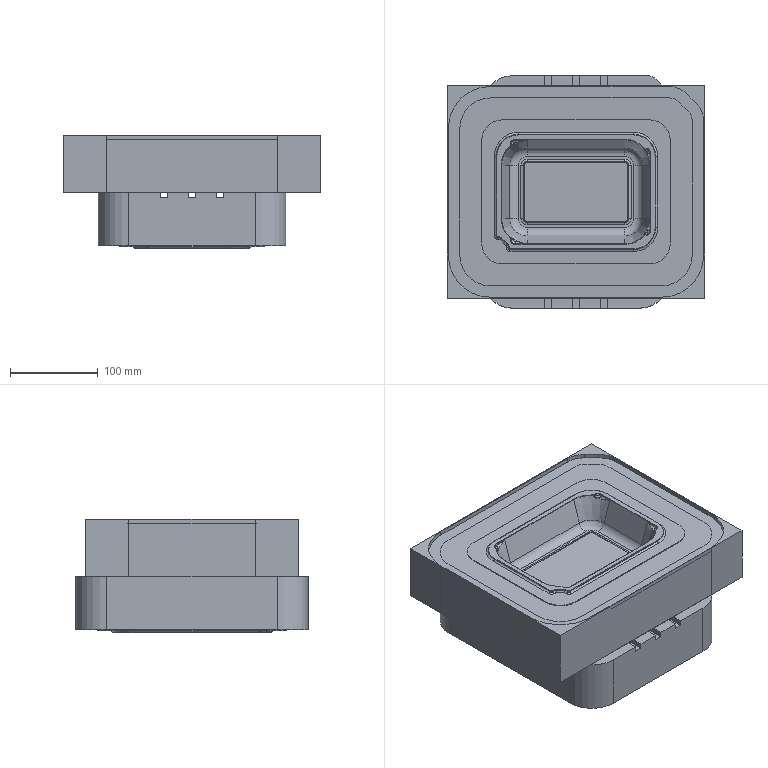NC program | NX | posted with a generic post | part box 293.342 x 265.342 x 129.5 mm
Lines 1 to 1156 of 68427:
N10 G17 G21 G94 G90
(B- , TOOL : D16R0.8)
N12 T00 M6
N14 G53
N16 G17 G0 G90 X-27.032 Y112.083 S7000 M3 M8
N18 G43 Z215.5 H0
N20 Z66.5
N22 G94 G1 X0. Z65.083 F4500.
N24 X106.458
N26 G2 X120.474 Y106.277 R19.822
N28 G1 X131.688 Y95.064
N30 G2 X137.493 Y81.047 R19.822
N32 G1 Y-72.26
N34 G2 X97.671 Y-112.083 R39.822
N36 G1 X-97.671
N38 G2 X-137.493 Y-72.26 R39.822
N40 G1 Y72.26
N42 G2 X-97.671 Y112.083 R39.822
N44 G1 X0.
N46 Y102.003
N48 X106.458
N50 G2 X113.347 Y99.149 R9.742
N52 G1 X124.56 Y87.936
N54 G2 X127.413 Y81.047 R9.742
N56 G1 Y-72.26
N58 G2 X97.671 Y-102.003 R29.742
N60 G1 X-97.671
N62 G2 X-127.413 Y-72.26 R29.742
N64 G1 Y72.26
N66 G2 X-97.671 Y102.003 R29.742
N68 G1 X0.
N70 Y91.923
N72 X106.318
N74 X117.333 Y80.907
N76 Y-72.262
N78 G2 X97.671 Y-91.923 R19.662
N80 G1 X-97.671
N82 G2 X-117.333 Y-72.26 R19.662
N84 G1 Y72.26
N86 G2 X-97.671 Y91.923 R19.662
N88 G1 X0.
N90 Y81.843
N92 X102.143
N94 X107.253 Y76.732
N96 Y-72.262
N98 G2 X97.671 Y-81.843 R9.582
N100 G1 X-97.671
N102 G2 X-107.253 Y-72.26 R9.582
N104 G1 Y72.26
N106 G2 X-97.671 Y81.843 R9.582
N108 G1 X0.
N110 Y71.763
N112 X97.173
N114 Y-71.763
N116 X-97.173
N118 Y71.763
N120 X0.
N122 Y61.683
N124 X87.093
N126 Y-61.683
N128 X-87.093
N130 Y61.683
N132 X0.
N134 Y51.603
N136 X77.013
N138 Y-51.603
N140 X-77.013
N142 Y51.603
N144 X0.
N146 Y41.523
N148 X66.933
N150 Y-41.523
N152 X-66.933
N154 Y41.523
N156 X0.
N158 Y31.443
N160 X56.853
N162 Y-31.443
N164 X-56.853
N166 Y31.443
N168 X0.
N170 Y21.363
N172 X46.773
N174 Y-21.363
N176 X-46.773
N178 Y21.363
N180 X0.
N182 Y11.283
N184 X36.693
N186 Y-11.283
N188 X-36.693
N190 Y11.283
N192 X0.
N194 Y1.203
N196 X26.613
N198 Y-1.203
N200 X-26.613
N202 Y1.203
N204 X0.
N206 G3 X3.2 Y4.403 R3.2
N208 G1 Z66.083
N210 G0 Z68.5
N212 X-27.032 Y112.01
N214 Z66.083
N216 G1 X0. Z64.667
N218 X106.458
N220 G2 X120.423 Y106.226 R19.75
N222 G1 X131.636 Y95.012
N224 G2 X137.421 Y81.047 R19.75
N226 G1 Y-72.26
N228 G2 X97.671 Y-112.01 R39.75
N230 G1 X-97.671
N232 G2 X-137.421 Y-72.26 R39.75
N234 G1 Y72.26
N236 G2 X-97.671 Y112.01 R39.75
N238 G1 X0.
N240 Y101.93
N242 X106.458
N244 G2 X113.296 Y99.098 R9.67
N246 G1 X124.509 Y87.885
N248 G2 X127.341 Y81.047 R9.67
N250 G1 Y-72.26
N252 G2 X97.671 Y-101.93 R29.67
N254 G1 X-97.671
N256 G2 X-127.341 Y-72.26 R29.67
N258 G1 Y72.26
N260 G2 X-97.671 Y101.93 R29.67
N262 G1 X0.
N264 Y91.85
N266 X106.288
N268 X117.261 Y80.877
N270 Y-72.26
N272 G2 X97.671 Y-91.85 R19.59
N274 G1 X-97.671
N276 G2 X-117.261 Y-72.26 R19.59
N278 G1 Y72.26
N280 G2 X-97.671 Y91.85 R19.59
N282 G1 X0.
N284 Y81.77
N286 X102.113
N288 X107.181 Y76.702
N290 Y-72.26
N292 G2 X97.671 Y-81.77 R9.51
N294 G1 X-97.671
N296 G2 X-107.181 Y-72.26 R9.51
N298 G1 Y72.26
N300 G2 X-97.671 Y81.77 R9.51
N302 G1 X0.
N304 Y71.69
N306 X97.101
N308 Y-71.69
N310 X-97.101
N312 Y71.69
N314 X0.
N316 Y61.61
N318 X87.021
N320 Y-61.61
N322 X-87.021
N324 Y61.61
N326 X0.
N328 Y51.53
N330 X76.941
N332 Y-51.53
N334 X-76.941
N336 Y51.53
N338 X0.
N340 Y41.45
N342 X66.861
N344 Y-41.45
N346 X-66.861
N348 Y41.45
N350 X0.
N352 Y31.37
N354 X56.781
N356 Y-31.37
N358 X-56.781
N360 Y31.37
N362 X0.
N364 Y21.29
N366 X46.701
N368 Y-21.29
N370 X-46.701
N372 Y21.29
N374 X0.
N376 Y11.21
N378 X36.621
N380 Y-11.21
N382 X-36.621
N384 Y11.21
N386 X0.
N388 Y1.13
N390 X26.541
N392 Y-1.13
N394 X-26.541
N396 Y1.13
N398 X0.
N400 G3 X3.2 Y4.33 R3.2
N402 G1 Z65.667
N404 G0 Z68.083
N406 X-27.032 Y112.01
N408 Z65.667
N410 G1 X0. Z64.25
N412 X106.458
N414 G2 X120.423 Y106.226 R19.75
N416 G1 X131.636 Y95.012
N418 G2 X137.421 Y81.047 R19.75
N420 G1 Y-72.26
N422 G2 X97.671 Y-112.01 R39.75
N424 G1 X-97.671
N426 G2 X-137.421 Y-72.26 R39.75
N428 G1 Y72.26
N430 G2 X-97.671 Y112.01 R39.75
N432 G1 X0.
N434 Y101.93
N436 X106.458
N438 G2 X113.296 Y99.098 R9.67
N440 G1 X124.509 Y87.885
N442 G2 X127.341 Y81.047 R9.67
N444 G1 Y-72.26
N446 G2 X97.671 Y-101.93 R29.67
N448 G1 X-97.671
N450 G2 X-127.341 Y-72.26 R29.67
N452 G1 Y72.26
N454 G2 X-97.671 Y101.93 R29.67
N456 G1 X0.
N458 Y91.85
N460 X106.288
N462 X117.261 Y80.877
N464 Y-72.26
N466 G2 X97.671 Y-91.85 R19.59
N468 G1 X-97.671
N470 G2 X-117.261 Y-72.26 R19.59
N472 G1 Y72.26
N474 G2 X-97.671 Y91.85 R19.59
N476 G1 X0.
N478 Y81.77
N480 X102.113
N482 X107.181 Y76.702
N484 Y-72.26
N486 G2 X97.671 Y-81.77 R9.51
N488 G1 X-97.671
N490 G2 X-107.181 Y-72.26 R9.51
N492 G1 Y72.26
N494 G2 X-97.671 Y81.77 R9.51
N496 G1 X0.
N498 Y71.69
N500 X97.101
N502 Y-71.69
N504 X-97.101
N506 Y71.69
N508 X0.
N510 Y61.61
N512 X87.021
N514 Y-61.61
N516 X-87.021
N518 Y61.61
N520 X0.
N522 Y51.53
N524 X76.941
N526 Y-51.53
N528 X-76.941
N530 Y51.53
N532 X0.
N534 Y41.45
N536 X66.861
N538 Y-41.45
N540 X-66.861
N542 Y41.45
N544 X0.
N546 Y31.37
N548 X56.781
N550 Y-31.37
N552 X-56.781
N554 Y31.37
N556 X0.
N558 Y21.29
N560 X46.701
N562 Y-21.29
N564 X-46.701
N566 Y21.29
N568 X0.
N570 Y11.21
N572 X36.621
N574 Y-11.21
N576 X-36.621
N578 Y11.21
N580 X0.
N582 Y1.13
N584 X26.541
N586 Y-1.13
N588 X-26.541
N590 Y1.13
N592 X0.
N594 G3 X3.2 Y4.33 R3.2
N596 G1 Z65.25
N598 G0 Z67.667
N600 X-26.516 Y112.01
N602 Z65.25
N604 G1 X0. Z63.86
N606 X106.458
N608 G2 X120.423 Y106.226 R19.75
N610 G1 X131.636 Y95.012
N612 G2 X137.421 Y81.047 R19.75
N614 G1 Y-72.26
N616 G2 X97.671 Y-112.01 R39.75
N618 G1 X-97.671
N620 G2 X-137.421 Y-72.26 R39.75
N622 G1 Y72.26
N624 G2 X-97.671 Y112.01 R39.75
N626 G1 X0.
N628 Y101.93
N630 X106.458
N632 G2 X113.296 Y99.098 R9.67
N634 G1 X124.509 Y87.885
N636 G2 X127.341 Y81.047 R9.67
N638 G1 Y-72.26
N640 G2 X97.671 Y-101.93 R29.67
N642 G1 X-97.671
N644 G2 X-127.341 Y-72.26 R29.67
N646 G1 Y72.26
N648 G2 X-97.671 Y101.93 R29.67
N650 G1 X0.
N652 Y91.85
N654 X106.288
N656 X117.261 Y80.877
N658 Y-72.26
N660 G2 X97.671 Y-91.85 R19.59
N662 G1 X-97.671
N664 G2 X-117.261 Y-72.26 R19.59
N666 G1 Y72.26
N668 G2 X-97.671 Y91.85 R19.59
N670 G1 X0.
N672 Y81.77
N674 X102.113
N676 X107.181 Y76.702
N678 Y55.718
N680 X97.101
N682 G3 X81.129 Y71.69 R34.895
N684 G1 X73.858 Y74.441
N686 X81.129 Y71.69
N688 X97.101
N690 Y55.718
N692 X99.852 Y48.447
N694 X97.101 Y55.718
N696 X107.181
N698 Y-72.26
N700 G2 X97.671 Y-81.77 R9.51
N702 G1 X81.129
N704 Y-71.69
N706 G3 X97.101 Y-55.718 R34.895
N708 G1 X99.852 Y-48.447
N710 X97.101 Y-55.718
N712 Y-71.69
N714 X81.129
N716 X73.858 Y-74.441
N718 X81.129 Y-71.69
N720 Y-81.77
N722 X-97.671
N724 G2 X-107.181 Y-72.26 R9.51
N726 G1 Y-58.072
N728 X-97.101
N730 G3 X-90.691 Y-61.119 R11.433
N732 G1 X-86.561 Y-65.248
N734 G3 X-83.48 Y-71.69 R11.5
N736 G1 X-97.101
N738 Y-58.072
N740 X-107.181
N742 Y72.26
N744 G2 X-97.671 Y81.77 R9.51
N746 G1 X-81.129
N748 Y71.69
N750 G3 X-97.101 Y55.718 R34.895
N752 G1 X-99.852 Y48.447
N754 X-97.101 Y55.718
N756 X-95.291 Y54.831
N758 G2 X-65.769 Y73.237 R32.879
N760 G1 X65.769
N762 G2 X98.648 Y40.358 R32.879
N764 G1 Y-40.358
N766 G2 X65.769 Y-73.237 R32.879
N768 G1 X-75.204
N770 G2 X-84.625 Y-64.333 R9.484
N772 G1 X-89.778 Y-59.181
N774 G2 X-98.648 Y-49.793 R9.417
N776 G1 Y40.358
N778 G2 X-95.291 Y54.831 R32.879
N780 G1 X-97.101 Y55.718
N782 Y71.69
N784 X-81.129
N786 X-73.858 Y74.441
N788 X-81.129 Y71.69
N790 Y81.77
N792 X0.
N794 G3 X3.2 Y84.97 R3.2
N796 G1 Z64.86
N798 G0 Z67.25
N800 X-26.516 Y112.01
N802 Z64.86
N804 G1 X0. Z63.471
N806 X106.458
N808 G2 X120.423 Y106.226 R19.75
N810 G1 X131.636 Y95.012
N812 G2 X137.421 Y81.047 R19.75
N814 G1 Y-72.26
N816 G2 X97.671 Y-112.01 R39.75
N818 G1 X-97.671
N820 G2 X-137.421 Y-72.26 R39.75
N822 G1 Y72.26
N824 G2 X-97.671 Y112.01 R39.75
N826 G1 X0.
N828 Y101.93
N830 X106.458
N832 G2 X113.296 Y99.098 R9.67
N834 G1 X124.509 Y87.885
N836 G2 X127.341 Y81.047 R9.67
N838 G1 Y-72.26
N840 G2 X97.671 Y-101.93 R29.67
N842 G1 X-97.671
N844 G2 X-127.341 Y-72.26 R29.67
N846 G1 Y72.26
N848 G2 X-97.671 Y101.93 R29.67
N850 G1 X0.
N852 Y91.85
N854 X106.288
N856 X117.261 Y80.877
N858 Y-72.26
N860 G2 X97.671 Y-91.85 R19.59
N862 G1 X-97.671
N864 G2 X-117.261 Y-72.26 R19.59
N866 G1 Y72.26
N868 G2 X-97.671 Y91.85 R19.59
N870 G1 X0.
N872 Y81.77
N874 X102.113
N876 X107.181 Y76.702
N878 Y56.426
N880 X97.101
N882 G3 X81.837 Y71.69 R35.212
N884 G1 X74.825 Y74.482
N886 X81.837 Y71.69
N888 X97.101
N890 Y56.426
N892 X99.893 Y49.414
N894 X97.101 Y56.426
N896 X107.181
N898 Y-72.26
N900 G2 X97.671 Y-81.77 R9.51
N902 G1 X81.837
N904 Y-71.69
N906 G3 X97.101 Y-56.426 R35.212
N908 G1 X99.893 Y-49.414
N910 X97.101 Y-56.426
N912 Y-71.69
N914 X81.837
N916 X74.825 Y-74.482
N918 X81.837 Y-71.69
N920 Y-81.77
N922 X-97.671
N924 G2 X-107.181 Y-72.26 R9.51
N926 G1 Y-58.514
N928 X-97.101
N930 G3 X-90.835 Y-61.423 R11.703
N932 G1 X-86.841 Y-65.417
N934 G3 X-83.924 Y-71.69 R11.718
N936 G1 X-97.101
N938 Y-58.514
N940 X-107.181
N942 Y72.26
N944 G2 X-97.671 Y81.77 R9.51
N946 G1 X-81.837
N948 Y71.69
N950 G3 X-97.101 Y56.426 R35.212
N952 G1 X-99.893 Y49.414
N954 X-97.101 Y56.426
N956 X-95.307 Y55.506
N958 G2 X-65.769 Y73.554 R33.196
N960 G1 X65.769
N962 G2 X98.965 Y40.358 R33.196
N964 G1 Y-40.358
N966 G2 X65.769 Y-73.554 R33.196
N968 G1 X-75.204
N970 X-75.261 Y-73.536
N972 G2 X-84.909 Y-64.498 R9.702
N974 G1 X-89.916 Y-59.491
N976 G2 X-98.947 Y-49.85 R9.687
N978 G1 X-98.965 Y-49.793
N980 Y40.358
N982 G2 X-95.307 Y55.506 R33.196
N984 G1 X-97.101 Y56.426
N986 Y71.69
N988 X-81.837
N990 X-74.825 Y74.482
N992 X-81.837 Y71.69
N994 Y81.77
N996 X0.
N998 G3 X3.2 Y84.97 R3.2
N1000 G1 Z64.471
N1002 G0 Z66.86
N1004 X-26.516 Y112.01
N1006 Z64.471
N1008 G1 X0. Z63.081
N1010 X106.458
N1012 G2 X120.423 Y106.226 R19.75
N1014 G1 X131.636 Y95.012
N1016 G2 X137.421 Y81.047 R19.75
N1018 G1 Y-72.26
N1020 G2 X97.671 Y-112.01 R39.75
N1022 G1 X-97.671
N1024 G2 X-137.421 Y-72.26 R39.75
N1026 G1 Y72.26
N1028 G2 X-97.671 Y112.01 R39.75
N1030 G1 X0.
N1032 Y101.93
N1034 X106.458
N1036 G2 X113.296 Y99.098 R9.67
N1038 G1 X124.509 Y87.885
N1040 G2 X127.341 Y81.047 R9.67
N1042 G1 Y-72.26
N1044 G2 X97.671 Y-101.93 R29.67
N1046 G1 X-97.671
N1048 G2 X-127.341 Y-72.26 R29.67
N1050 G1 Y72.26
N1052 G2 X-97.671 Y101.93 R29.67
N1054 G1 X0.
N1056 Y91.85
N1058 X106.288
N1060 X117.261 Y80.877
N1062 Y-72.26
N1064 G2 X97.671 Y-91.85 R19.59
N1066 G1 X-97.671
N1068 G2 X-117.261 Y-72.26 R19.59
N1070 G1 Y72.26
N1072 G2 X-97.671 Y91.85 R19.59
N1074 G1 X0.
N1076 Y81.77
N1078 X102.113
N1080 X107.181 Y76.702
N1082 Y56.786
N1084 X97.101
N1086 G3 X82.197 Y71.69 R35.378
N1088 G1 X75.297 Y74.503
N1090 X82.197 Y71.69
N1092 X97.101
N1094 Y56.786
N1096 X99.914 Y49.887
N1098 X97.101 Y56.786
N1100 X107.181
N1102 Y-72.26
N1104 G2 X97.671 Y-81.77 R9.51
N1106 G1 X82.197
N1108 Y-71.69
N1110 G3 X97.101 Y-56.786 R35.378
N1112 G1 X99.914 Y-49.887
N1114 X97.101 Y-56.786
N1116 Y-71.69
N1118 X82.197
N1120 X75.297 Y-74.503
N1122 X82.197 Y-71.69
N1124 Y-81.77
N1126 X-97.671
N1128 G2 X-107.181 Y-72.26 R9.51
N1130 G1 Y-58.792
N1132 X-97.101
N1134 G3 X-90.887 Y-61.606 R11.821
N1136 G1 X-87.01 Y-65.483
N1138 G3 X-84.207 Y-71.69 R11.798
N1140 G1 X-97.101
N1142 Y-58.792
N1144 X-107.181
N1146 Y72.26
N1148 G2 X-97.671 Y81.77 R9.51
N1150 G1 X-82.197
N1152 Y71.69
N1154 G3 X-97.101 Y56.786 R35.378
N1156 G1 X-99.914 Y49.887
N1158 X-97.101 Y56.786
N1160 X-95.316 Y55.85
N1162 G2 X-65.769 Y73.72 R33.362
N1164 G1 X65.769
N1166 G2 X99.131 Y40.358 R33.362
N1168 G1 Y-40.358
N1170 G2 X65.769 Y-73.72 R33.362
N1172 G1 X-75.258
N1174 G2 X-85.075 Y-64.566 R9.782
N1176 G1 X-89.97 Y-59.672
N1178 G2 X-99.131 Y-49.848 R9.805
N1180 G1 Y40.358
N1182 G2 X-95.316 Y55.85 R33.362
N1184 G1 X-97.101 Y56.786
N1186 Y71.69
N1188 X-82.197
N1190 X-75.297 Y74.503
N1192 X-82.197 Y71.69
N1194 Y81.77
N1196 X0.
N1198 G3 X3.2 Y84.97 R3.2
N1200 G1 Z64.081
N1202 G0 Z66.471
N1204 X-26.516 Y112.01
N1206 Z64.081
N1208 G1 X0. Z62.691
N1210 X106.458
N1212 G2 X120.423 Y106.226 R19.75
N1214 G1 X131.636 Y95.012
N1216 G2 X137.421 Y81.047 R19.75
N1218 G1 Y-72.26
N1220 G2 X97.671 Y-112.01 R39.75
N1222 G1 X-97.671
N1224 G2 X-137.421 Y-72.26 R39.75
N1226 G1 Y72.26
N1228 G2 X-97.671 Y112.01 R39.75
N1230 G1 X0.
N1232 Y101.93
N1234 X106.458
N1236 G2 X113.296 Y99.098 R9.67
N1238 G1 X124.509 Y87.885
N1240 G2 X127.341 Y81.047 R9.67
N1242 G1 Y-72.26
N1244 G2 X97.671 Y-101.93 R29.67
N1246 G1 X-97.671
N1248 G2 X-127.341 Y-72.26 R29.67
N1250 G1 Y72.26
N1252 G2 X-97.671 Y101.93 R29.67
N1254 G1 X0.
N1256 Y91.85
N1258 X106.288
N1260 X117.261 Y80.877
N1262 Y-72.26
N1264 G2 X97.671 Y-91.85 R19.59
N1266 G1 X-97.671
N1268 G2 X-117.261 Y-72.26 R19.59
N1270 G1 Y72.26
N1272 G2 X-97.671 Y91.85 R19.59
N1274 G1 X0.
N1276 Y81.77
N1278 X102.113
N1280 X107.181 Y76.702
N1282 Y57.118
N1284 X97.101
N1286 G3 X82.529 Y71.69 R35.533
N1288 G1 X75.723 Y74.522
N1290 X82.529 Y71.69
N1292 X97.101
N1294 Y57.118
N1296 X99.933 Y50.312
N1298 X97.101 Y57.118
N1300 X107.181
N1302 Y-72.26
N1304 G2 X97.671 Y-81.77 R9.51
N1306 G1 X82.529
N1308 Y-71.69
N1310 G3 X97.101 Y-57.118 R35.533
N1312 G1 X99.933 Y-50.312
N1314 X97.101 Y-57.118
N1316 Y-71.69
N1318 X82.529
N1320 X75.723 Y-74.522
N1322 X82.529 Y-71.69
N1324 Y-81.77
N1326 X-97.671
N1328 G2 X-107.181 Y-72.26 R9.51
N1330 G1 Y-59.071
N1332 X-97.101
N1334 G3 X-90.944 Y-61.769 R11.812
N1336 G1 X-87.174 Y-65.538
N1338 G3 X-84.483 Y-71.69 R11.797
N1340 G1 X-97.101
N1342 Y-59.071
N1344 X-107.181
N1346 Y72.26
N1348 G2 X-97.671 Y81.77 R9.51
N1350 G1 X-82.529
N1352 Y71.69
N1354 G3 X-97.101 Y57.118 R35.533
N1356 G1 X-99.933 Y50.312
N1358 X-97.101 Y57.118
N1360 X-95.323 Y56.167
N1362 G2 X-65.769 Y73.875 R33.517
N1364 G1 X65.769
N1366 G2 X99.286 Y40.358 R33.517
N1368 G1 Y-40.358
N1370 G2 X65.769 Y-73.875 R33.517
N1372 G1 X-75.755
N1374 G2 X-76.587 Y-73.799 R4.574
N1376 X-85.233 Y-64.628 R9.781
N1378 G1 X-90.033 Y-59.828
N1380 G2 X-99.211 Y-51.163 R9.796
N1382 X-99.286 Y-50.671 R1.653
N1384 G1 Y40.358
N1386 G2 X-95.323 Y56.167 R33.517
N1388 G1 X-97.101 Y57.118
N1390 Y71.69
N1392 X-82.529
N1394 X-75.723 Y74.522
N1396 X-82.529 Y71.69
N1398 Y81.77
N1400 X0.
N1402 G3 X3.2 Y84.97 R3.2
N1404 G1 Z63.691
N1406 G0 Z66.081
N1408 X-26.516 Y112.01
N1410 Z63.691
N1412 G1 X0. Z62.302
N1414 X106.458
N1416 G2 X120.423 Y106.226 R19.75
N1418 G1 X131.636 Y95.012
N1420 G2 X137.421 Y81.047 R19.75
N1422 G1 Y-72.26
N1424 G2 X97.671 Y-112.01 R39.75
N1426 G1 X-97.671
N1428 G2 X-137.421 Y-72.26 R39.75
N1430 G1 Y72.26
N1432 G2 X-97.671 Y112.01 R39.75
N1434 G1 X0.
N1436 Y101.93
N1438 X106.458
N1440 G2 X113.296 Y99.098 R9.67
N1442 G1 X124.509 Y87.885
N1444 G2 X127.341 Y81.047 R9.67
N1446 G1 Y-72.26
N1448 G2 X97.671 Y-101.93 R29.67
N1450 G1 X-97.671
N1452 G2 X-127.341 Y-72.26 R29.67
N1454 G1 Y72.26
N1456 G2 X-97.671 Y101.93 R29.67
N1458 G1 X0.
N1460 Y91.85
N1462 X106.288
N1464 X117.261 Y80.877
N1466 Y-72.26
N1468 G2 X97.671 Y-91.85 R19.59
N1470 G1 X-97.671
N1472 G2 X-117.261 Y-72.26 R19.59
N1474 G1 Y72.26
N1476 G2 X-97.671 Y91.85 R19.59
N1478 G1 X0.
N1480 Y81.77
N1482 X102.113
N1484 X107.181 Y76.702
N1486 Y57.738
N1488 X97.101
N1490 G3 X83.149 Y71.69 R35.829
N1492 G1 X76.499 Y74.558
N1494 X83.149 Y71.69
N1496 X97.101
N1498 Y57.738
N1500 X99.968 Y51.088
N1502 X97.101 Y57.738
N1504 X107.181
N1506 Y-72.26
N1508 G2 X97.671 Y-81.77 R9.51
N1510 G1 X83.149
N1512 Y-71.69
N1514 G3 X97.101 Y-57.738 R35.829
N1516 G1 X99.968 Y-51.088
N1518 X97.101 Y-57.738
N1520 Y-71.69
N1522 X83.149
N1524 X76.499 Y-74.558
N1526 X83.149 Y-71.69
N1528 Y-81.77
N1530 X-97.671
N1532 G2 X-107.181 Y-72.26 R9.51
N1534 G1 Y-59.468
N1536 X-97.101
N1538 G3 X-91.078 Y-62.054 R12.108
N1540 G1 X-87.461 Y-65.67
N1542 G3 X-84.877 Y-71.69 R12.104
N1544 G1 X-97.101
N1546 Y-59.468
N1548 X-107.181
N1550 Y72.26
N1552 G2 X-97.671 Y81.77 R9.51
N1554 G1 X-83.149
N1556 Y71.69
N1558 G3 X-97.101 Y57.738 R35.829
N1560 G1 X-99.968 Y51.088
N1562 X-97.101 Y57.738
N1564 X-95.338 Y56.76
N1566 G2 X-65.769 Y74.172 R33.813
N1568 G1 X65.769
N1570 G2 X99.582 Y40.358 R33.813
N1572 G1 Y-40.358
N1574 G2 X65.769 Y-74.172 R33.813
N1576 G1 X-75.337
N1578 G2 X-85.528 Y-64.753 R10.088
N1580 G1 X-90.161 Y-60.12
N1582 G2 X-99.582 Y-49.926 R10.092
N1584 G1 Y40.358
N1586 G2 X-95.338 Y56.76 R33.813
N1588 G1 X-97.101 Y57.738
N1590 Y71.69
N1592 X-83.149
N1594 X-76.499 Y74.558
N1596 X-83.149 Y71.69
N1598 Y81.77
N1600 X0.
N1602 G3 X3.2 Y84.97 R3.2
N1604 G1 Z63.302
N1606 G0 Z65.691
N1608 X-26.516 Y112.01
N1610 Z63.302
N1612 G1 X0. Z61.912
N1614 X106.458
N1616 G2 X120.423 Y106.226 R19.75
N1618 G1 X131.636 Y95.012
N1620 G2 X137.421 Y81.047 R19.75
N1622 G1 Y-72.26
N1624 G2 X97.671 Y-112.01 R39.75
N1626 G1 X-97.671
N1628 G2 X-137.421 Y-72.26 R39.75
N1630 G1 Y72.26
N1632 G2 X-97.671 Y112.01 R39.75
N1634 G1 X0.
N1636 Y101.93
N1638 X106.458
N1640 G2 X113.296 Y99.098 R9.67
N1642 G1 X124.509 Y87.885
N1644 G2 X127.341 Y81.047 R9.67
N1646 G1 Y-72.26
N1648 G2 X97.671 Y-101.93 R29.67
N1650 G1 X-97.671
N1652 G2 X-127.341 Y-72.26 R29.67
N1654 G1 Y72.26
N1656 G2 X-97.671 Y101.93 R29.67
N1658 G1 X0.
N1660 Y91.85
N1662 X106.288
N1664 X117.261 Y80.877
N1666 Y-72.26
N1668 G2 X97.671 Y-91.85 R19.59
N1670 G1 X-97.671
N1672 G2 X-117.261 Y-72.26 R19.59
N1674 G1 Y72.26
N1676 G2 X-97.671 Y91.85 R19.59
N1678 G1 X0.
N1680 Y81.77
N1682 X102.113
N1684 X107.181 Y76.702
N1686 Y59.413
N1688 X97.101
N1690 G3 X84.824 Y71.69 R36.671
N1692 G1 X97.101
N1694 Y59.413
N1696 X107.181
N1698 Y-72.26
N1700 G2 X97.671 Y-81.77 R9.51
N1702 G1 X84.824
N1704 Y-71.69
N1706 G3 X97.101 Y-59.413 R36.671
N1708 G1 Y-71.69
N1710 X84.824
N1712 Y-81.77
N1714 X-97.671
N1716 G2 X-107.181 Y-72.26 R9.51
N1718 G1 Y-60.654
N1720 X-97.101
N1722 G3 X-91.375 Y-62.947 R12.832
N1724 G1 X-88.382 Y-65.94
N1726 G3 X-86.067 Y-71.69 R12.885
N1728 G1 X-97.101
N1730 Y-60.654
N1732 X-107.181
N1734 Y72.26
N1736 G2 X-97.671 Y81.77 R9.51
N1738 G1 X-84.824
N1740 Y71.69
N1742 G3 X-97.101 Y59.413 R36.671
N1744 G1 X-95.379 Y58.365
N1746 G2 X-65.769 Y75.013 R34.655
N1748 G1 X65.769
N1750 G2 X100.424 Y40.358 R34.655
N1752 G1 Y-40.358
N1754 G2 X65.769 Y-75.013 R34.655
N1756 G1 X-75.623
N1758 G2 X-86.457 Y-65.014 R10.869
N1760 G1 X-90.451 Y-61.02
N1762 G2 X-100.424 Y-50.237 R10.816
N1764 G1 Y40.358
N1766 G2 X-95.379 Y58.365 R34.655
N1768 G1 X-97.101 Y59.413
N1770 Y71.69
N1772 X-84.824
N1774 Y81.77
N1776 X0.
N1778 G3 X3.2 Y84.97 R3.2
N1780 G1 Z62.912
N1782 G0 Z65.302
N1784 X-25.197 Y112.01
N1786 Z62.912
N1788 G1 X0. Z61.592
N1790 X106.458
N1792 G2 X120.423 Y106.226 R19.75
N1794 G1 X131.636 Y95.012
N1796 G2 X137.421 Y81.047 R19.75
N1798 G1 Y-72.26
N1800 G2 X97.671 Y-112.01 R39.75
N1802 G1 X-97.671
N1804 G2 X-137.421 Y-72.26 R39.75
N1806 G1 Y72.26
N1808 G2 X-97.671 Y112.01 R39.75
N1810 G1 X0.
N1812 Y101.93
N1814 X106.458
N1816 G2 X113.296 Y99.098 R9.67
N1818 G1 X124.509 Y87.885
N1820 G2 X127.341 Y81.047 R9.67
N1822 G1 Y63.335
N1824 X117.261
N1826 G3 X88.746 Y91.85 R33.971
N1828 G1 X106.288
N1830 X117.261 Y80.877
N1832 Y63.335
N1834 X117.642 Y56.145
N1836 Y-56.145
N1838 G2 X120.141 Y-56.736 R7.2
N1840 G1 Y56.736
N1842 G2 X117.642 Y56.145 R7.2
N1844 G1 X117.261 Y63.335
N1846 X127.341
N1848 Y-72.26
N1850 G2 X97.671 Y-101.93 R29.67
N1852 G1 X88.746
N1854 Y-91.85
N1856 G3 X117.261 Y-63.335 R33.971
N1858 G1 Y-72.26
N1860 G2 X97.671 Y-91.85 R19.59
N1862 G1 X88.746
N1864 Y-101.93
N1866 X-97.671
N1868 G2 X-127.341 Y-72.26 R29.67
N1870 G1 Y-63.335
N1872 X-117.261
N1874 G3 X-88.746 Y-91.85 R33.971
N1876 G1 X-82.147 Y-94.73
N1878 X82.147
N1880 G2 X81.556 Y-92.231 R7.2
N1882 G1 X-81.556
N1884 G2 X-82.147 Y-94.73 R7.2
N1886 G1 X-88.746 Y-91.85
N1888 X-97.671
N1890 G2 X-117.261 Y-72.26 R19.59
N1892 G1 Y-63.335
N1894 X-117.642 Y-56.145
N1896 Y56.145
N1898 G2 X-120.141 Y56.736 R7.2
N1900 G1 Y-56.736
N1902 G2 X-117.642 Y-56.145 R7.2
N1904 G1 X-117.261 Y-63.335
N1906 X-127.341
N1908 Y72.26
N1910 G2 X-97.671 Y101.93 R29.67
N1912 G1 X-88.746
N1914 Y91.85
N1916 G3 X-117.261 Y63.335 R33.971
N1918 G1 X-115.268 Y63.034
N1920 G2 X-83.671 Y90.215 R31.955
N1922 G1 X83.671
N1924 G2 X115.626 Y58.26 R31.955
N1926 G1 Y-58.26
N1928 G2 X83.671 Y-90.215 R31.955
N1930 G1 X-83.671
N1932 G2 X-115.626 Y-58.26 R31.955
N1934 G1 Y58.26
N1936 G2 X-115.268 Y63.034 R31.955
N1938 G1 X-117.261 Y63.335
N1940 Y72.26
N1942 G2 X-97.671 Y91.85 R19.59
N1944 G1 X-88.746
N1946 X-81.556 Y92.231
N1948 X81.556
N1950 G2 X82.147 Y94.73 R7.2
N1952 G1 X-82.147
N1954 G2 X-81.556 Y92.231 R7.2
N1956 G1 X-88.746 Y91.85
N1958 Y101.93
N1960 X0.
N1962 G3 X3.2 Y105.13 R3.2
N1964 G1 Z62.592
N1966 G0 Z64.912
N1968 X-25.197 Y112.01
N1970 Z62.592
N1972 G1 X0. Z61.271
N1974 X106.458
N1976 G2 X120.423 Y106.226 R19.75
N1978 G1 X131.636 Y95.012
N1980 G2 X137.421 Y81.047 R19.75
N1982 G1 Y-72.26
N1984 G2 X97.671 Y-112.01 R39.75
N1986 G1 X-97.671
N1988 G2 X-137.421 Y-72.26 R39.75
N1990 G1 Y72.26
N1992 G2 X-97.671 Y112.01 R39.75
N1994 G1 X0.
N1996 Y101.93
N1998 X106.458
N2000 G2 X113.296 Y99.098 R9.67
N2002 G1 X124.509 Y87.885
N2004 G2 X127.341 Y81.047 R9.67
N2006 G1 Y64.6
N2008 X117.261
N2010 G3 X90.011 Y91.85 R34.183
N2012 G1 X106.288
N2014 X117.261 Y80.877
N2016 Y64.6
N2018 X117.854 Y57.425
N2020 Y-57.425
N2022 G2 X120.141 Y-58.001 R7.2
N2024 G1 Y58.001
N2026 G2 X117.854 Y57.425 R7.2
N2028 G1 X117.261 Y64.6
N2030 X127.341
N2032 Y-72.26
N2034 G2 X97.671 Y-101.93 R29.67
N2036 G1 X90.011
N2038 Y-91.85
N2040 G3 X117.261 Y-64.6 R34.183
N2042 G1 Y-72.26
N2044 G2 X97.671 Y-91.85 R19.59
N2046 G1 X90.011
N2048 Y-101.93
N2050 X-97.671
N2052 G2 X-127.341 Y-72.26 R29.67
N2054 G1 Y-64.6
N2056 X-117.261
N2058 G3 X-90.011 Y-91.85 R34.183
N2060 G1 X-83.412 Y-94.73
N2062 X83.412
N2064 G2 X82.835 Y-92.443 R7.2
N2066 G1 X-82.835
N2068 G2 X-83.412 Y-94.73 R7.2
N2070 G1 X-90.011 Y-91.85
N2072 X-97.671
N2074 G2 X-117.261 Y-72.26 R19.59
N2076 G1 Y-64.6
N2078 X-117.854 Y-57.425
N2080 Y57.425
N2082 G2 X-120.141 Y58.001 R7.2
N2084 G1 Y-58.001
N2086 G2 X-117.854 Y-57.425 R7.2
N2088 G1 X-117.261 Y-64.6
N2090 X-127.341
N2092 Y72.26
N2094 G2 X-97.671 Y101.93 R29.67
N2096 G1 X-90.011
N2098 Y91.85
N2100 G3 X-117.261 Y64.6 R34.183
N2102 G1 X-115.28 Y64.226
N2104 G2 X-83.671 Y90.427 R32.167
N2106 G1 X83.671
N2108 G2 X115.838 Y58.26 R32.167
N2110 G1 Y-58.26
N2112 G2 X83.671 Y-90.427 R32.167
N2114 G1 X-83.671
N2116 G2 X-115.838 Y-58.26 R32.167
N2118 G1 Y58.26
N2120 G2 X-115.28 Y64.226 R32.167
N2122 G1 X-117.261 Y64.6
N2124 Y72.26
N2126 G2 X-97.671 Y91.85 R19.59
N2128 G1 X-90.011
N2130 X-82.835 Y92.443
N2132 X82.835
N2134 G2 X83.412 Y94.73 R7.2
N2136 G1 X-83.412
N2138 G2 X-82.835 Y92.443 R7.2
N2140 G1 X-90.011 Y91.85
N2142 Y101.93
N2144 X0.
N2146 G3 X3.2 Y105.13 R3.2
N2148 G1 Z62.271
N2150 G0 Z64.592
N2152 X72.431 Y112.01
N2154 Z62.271
N2156 G1 X98.362 Z60.912
N2158 X106.458
N2160 G2 X120.423 Y106.226 R19.75
N2162 G1 X131.636 Y95.012
N2164 G2 X137.421 Y81.047 R19.75
N2166 G1 Y-72.26
N2168 G2 X97.671 Y-112.01 R39.75
N2170 G1 X-97.671
N2172 G2 X-137.421 Y-72.26 R39.75
N2174 G1 Y72.26
N2176 G2 X-97.671 Y112.01 R39.75
N2178 G1 X98.362
N2180 Y101.93
N2182 X106.458
N2184 G2 X113.296 Y99.098 R9.67
N2186 G1 X124.509 Y87.885
N2188 G2 X127.341 Y81.047 R9.67
N2190 G1 Y-72.26
N2192 G2 X97.671 Y-101.93 R29.67
N2194 G1 X90.436
N2196 Y-91.85
N2198 G3 X117.261 Y-65.025 R34.264
N2200 G1 Y-72.26
N2202 G2 X97.671 Y-91.85 R19.59
N2204 G1 X90.436
N2206 Y-101.93
N2208 X-97.671
N2210 G2 X-127.341 Y-72.26 R29.67
N2212 G1 Y-65.025
N2214 X-117.261
N2216 G3 X-90.436 Y-91.85 R34.264
N2218 G1 X-83.837 Y-94.73
N2220 X83.837
N2222 G2 X83.267 Y-92.525 R7.2
N2224 G1 X-83.267
N2226 G2 X-83.837 Y-94.73 R7.2
N2228 G1 X-90.436 Y-91.85
N2230 X-97.671
N2232 G2 X-117.261 Y-72.26 R19.59
N2234 G1 Y-65.025
N2236 X-117.935 Y-57.857
N2238 Y57.857
N2240 G2 X-120.141 Y58.426 R7.2
N2242 G1 Y-58.426
N2244 G2 X-117.935 Y-57.857 R7.2
N2246 G1 X-117.261 Y-65.025
N2248 X-127.341
N2250 Y72.26
N2252 G2 X-97.671 Y101.93 R29.67
N2254 G1 X-90.436
N2256 Y91.85
N2258 G3 X-117.261 Y65.025 R34.264
N2260 G1 Y72.26
N2262 G2 X-97.671 Y91.85 R19.59
N2264 G1 X-90.436
N2266 X-83.267 Y92.525
N2268 X83.267
N2270 G2 X83.837 Y94.73 R7.2
N2272 G1 X-83.837
N2274 G2 X-83.267 Y92.525 R7.2
N2276 G1 X-90.436 Y91.85
N2278 Y101.93
N2280 X98.362
N2282 Y91.85
N2284 X106.288
N2286 X117.261 Y80.877
N2288 Y65.025
N2290 X117.935 Y57.857
N2292 Y-57.857
N2294 G2 X120.141 Y-58.426 R7.2
N2296 G1 Y58.426
N2298 G2 X117.935 Y57.857 R7.2
N2300 G1 X117.261 Y65.025
N2302 G3 X90.436 Y91.85 R34.264
N2304 G1 X90.038 Y89.874
N2306 G2 X115.919 Y58.26 R32.248
N2308 G1 Y-58.26
N2310 G2 X83.671 Y-90.509 R32.248